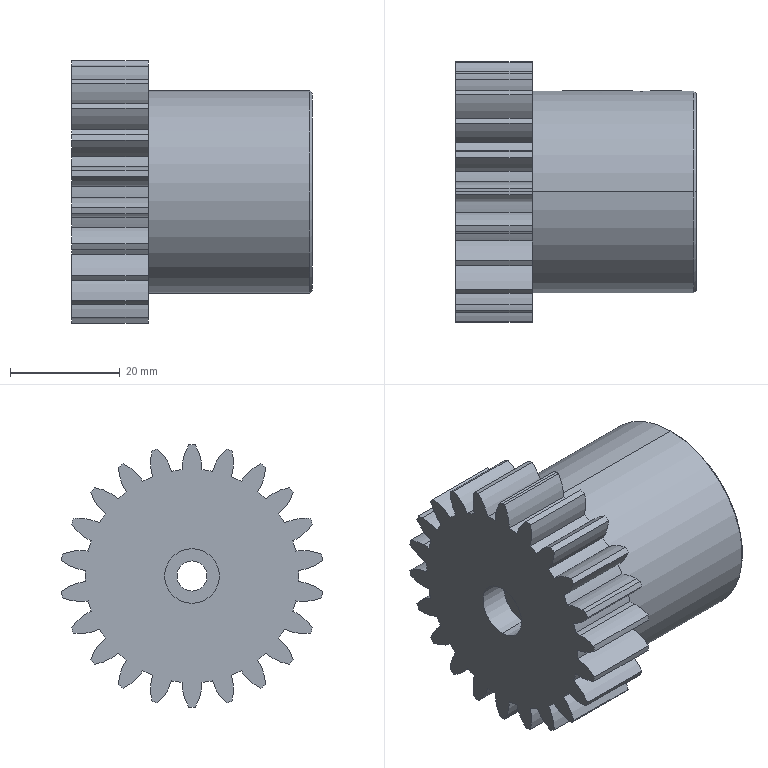Part | SolidWorks | features ICE 5, HoleWzd 4, BaseBody 1, Chamfer 1, RevCut 1 | 1 solid | 117 faces | box 44 x 47.656 x 48 mm | volume 38750 mm3 | cylinder 104 | plane 8 | cone 5 | commonest cylinder face diameters 17.6 x48 48 x23 38.998 x22 22 x3 4.2 x2 5.5 x2